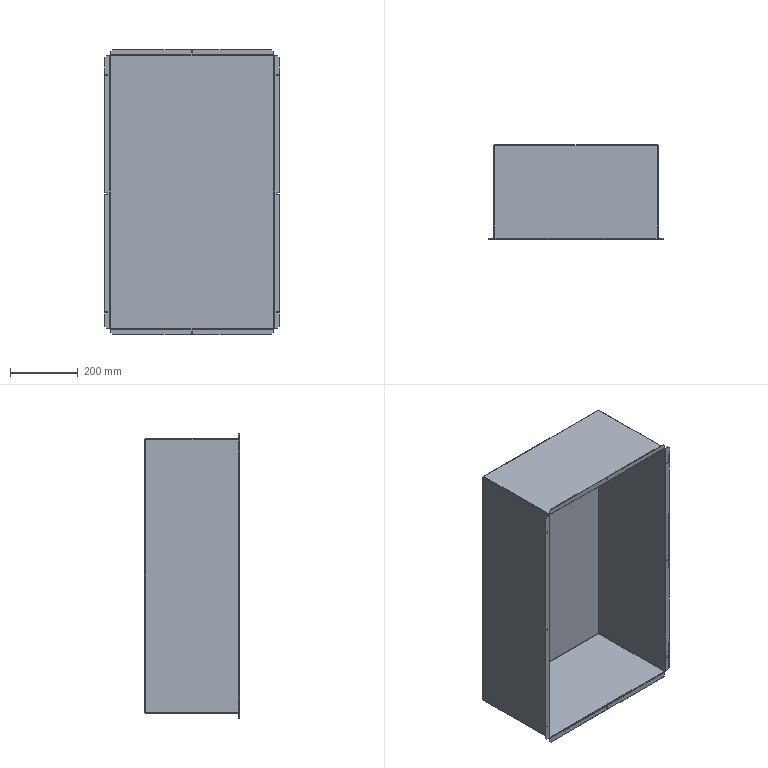Part | NX | 1 solid | 110 faces | box 515 x 278 x 840 mm | volume 2274406 mm3 | plane 78 | cylinder 24 | spline 8 | commonest cylinder face diameters 0.4 x8 4.3 x8 4.4 x8